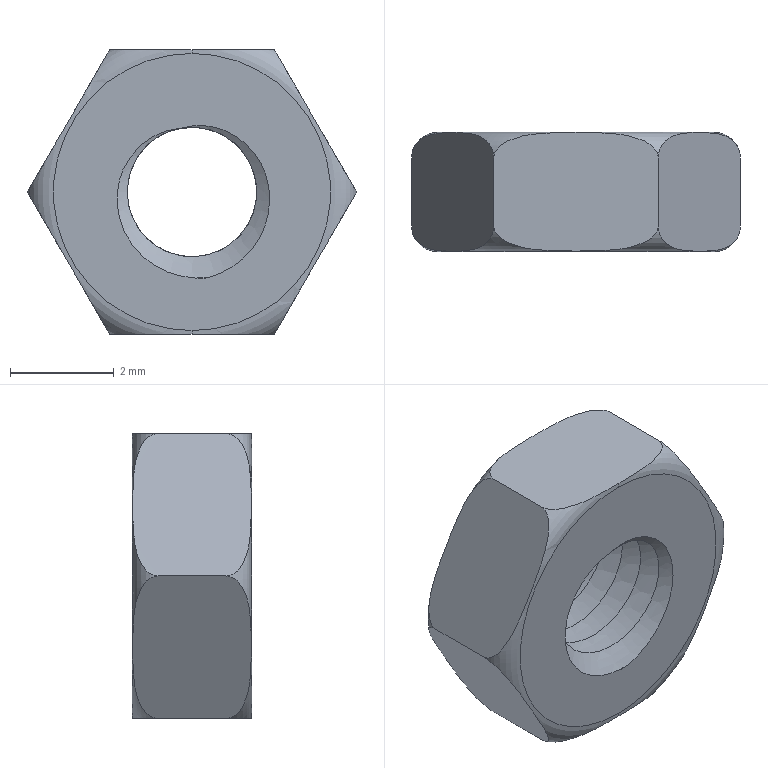Part | STEP file | AD-3MM-2_1_2.stp | 1 solid | 14 faces | volume 44.135 mm3 | plane 8 | torus 4 | spline 2